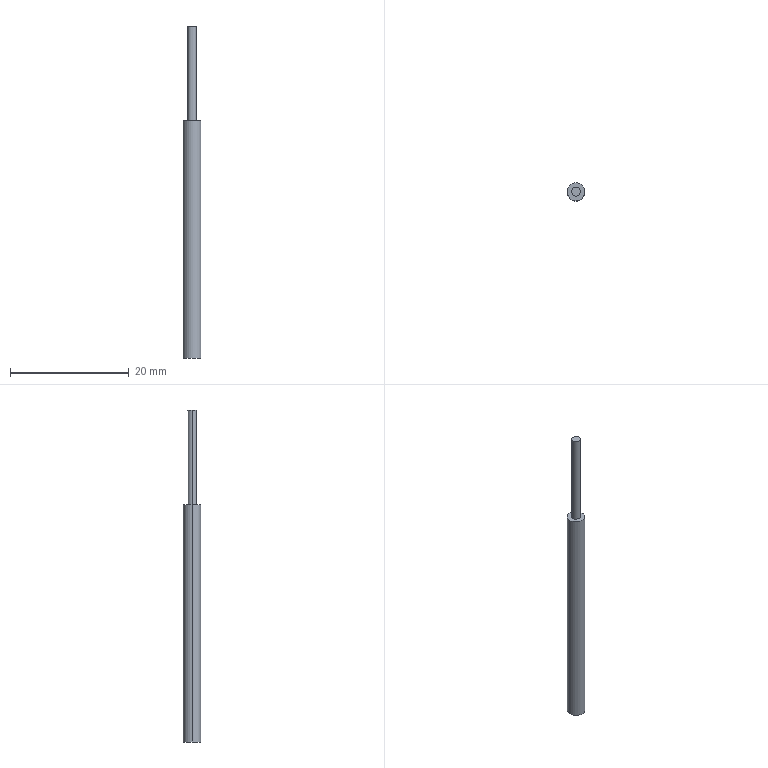Part | SolidWorks | features Extrusion 1, ICE 1 | 1 solid | 7 faces | box 3 x 3 x 56 mm | volume 311.018 mm3 | cylinder 4 | plane 3 | commonest cylinder face diameters 1.5 x2 3 x2
STEP:
#1=CARTESIAN_POINT('',(0.75,0.,56.));
#2=VERTEX_POINT('',#1);
#3=CARTESIAN_POINT('',(-0.75,0.,56.));
#4=VERTEX_POINT('',#3);
#5=CARTESIAN_POINT('',(0.,0.,56.));
#6=DIRECTION('',(0.,0.,1.));
#7=DIRECTION('',(1.,0.,0.));
#8=AXIS2_PLACEMENT_3D('',#5,#6,#7);
#9=CIRCLE('',#8,0.75);
#10=EDGE_CURVE('',#2,#4,#9,.T.);
#11=ORIENTED_EDGE('',*,*,#10,.F.);
#12=CARTESIAN_POINT('',(0.75,0.,40.));
#13=VERTEX_POINT('',#12);
#14=CARTESIAN_POINT('',(0.75,0.,56.));
#15=DIRECTION('',(0.,0.,-1.));
#16=VECTOR('',#15,1000.);
#17=LINE('',#14,#16);
#18=EDGE_CURVE('',#2,#13,#17,.T.);
#19=ORIENTED_EDGE('',*,*,#18,.T.);
#20=CARTESIAN_POINT('',(-0.75,0.,40.));
#21=VERTEX_POINT('',#20);
#22=CARTESIAN_POINT('',(0.,0.,40.));
#23=DIRECTION('',(0.,0.,1.));
#24=DIRECTION('',(1.,0.,0.));
#25=AXIS2_PLACEMENT_3D('',#22,#23,#24);
#26=CIRCLE('',#25,0.75);
#27=EDGE_CURVE('',#13,#21,#26,.T.);
#28=ORIENTED_EDGE('',*,*,#27,.T.);
#29=CARTESIAN_POINT('',(-0.75,0.,56.));
#30=DIRECTION('',(0.,0.,-1.));
#31=VECTOR('',#30,1000.);
#32=LINE('',#29,#31);
#33=EDGE_CURVE('',#4,#21,#32,.T.);
#34=ORIENTED_EDGE('',*,*,#33,.F.);
#35=EDGE_LOOP('',(#11,#19,#28,#34));
#36=FACE_OUTER_BOUND('',#35,.T.);
#37=CARTESIAN_POINT('',(0.,0.,56.));
#38=DIRECTION('',(0.,0.,-1.));
#39=DIRECTION('',(-1.,0.,0.));
#40=AXIS2_PLACEMENT_3D('',#37,#38,#39);
#41=CYLINDRICAL_SURFACE('',#40,0.75);
#42=ADVANCED_FACE('',(#36),#41,.T.);
#43=CARTESIAN_POINT('',(1.5,0.,40.));
#44=VERTEX_POINT('',#43);
#45=CARTESIAN_POINT('',(-1.5,0.,40.));
#46=VERTEX_POINT('',#45);
#47=CARTESIAN_POINT('',(0.,0.,40.));
#48=DIRECTION('',(0.,0.,1.));
#49=DIRECTION('',(1.,0.,0.));
#50=AXIS2_PLACEMENT_3D('',#47,#48,#49);
#51=CIRCLE('',#50,1.5);
#52=EDGE_CURVE('',#44,#46,#51,.T.);
#53=ORIENTED_EDGE('',*,*,#52,.F.);
#54=CARTESIAN_POINT('',(1.5,0.,0.));
#55=VERTEX_POINT('',#54);
#56=CARTESIAN_POINT('',(1.5,0.,40.));
#57=DIRECTION('',(0.,0.,-1.));
#58=VECTOR('',#57,1000.);
#59=LINE('',#56,#58);
#60=EDGE_CURVE('',#44,#55,#59,.T.);
#61=ORIENTED_EDGE('',*,*,#60,.T.);
#62=CARTESIAN_POINT('',(-1.5,0.,0.));
#63=VERTEX_POINT('',#62);
#64=CARTESIAN_POINT('',(0.,0.,0.));
#65=DIRECTION('',(0.,0.,1.));
#66=DIRECTION('',(1.,0.,0.));
#67=AXIS2_PLACEMENT_3D('',#64,#65,#66);
#68=CIRCLE('',#67,1.5);
#69=EDGE_CURVE('',#55,#63,#68,.T.);
#70=ORIENTED_EDGE('',*,*,#69,.T.);
#71=CARTESIAN_POINT('',(-1.5,0.,40.));
#72=DIRECTION('',(0.,0.,-1.));
#73=VECTOR('',#72,1000.);
#74=LINE('',#71,#73);
#75=EDGE_CURVE('',#46,#63,#74,.T.);
#76=ORIENTED_EDGE('',*,*,#75,.F.);
#77=EDGE_LOOP('',(#53,#61,#70,#76));
#78=FACE_OUTER_BOUND('',#77,.T.);
#79=CARTESIAN_POINT('',(0.,0.,40.));
#80=DIRECTION('',(0.,0.,-1.));
#81=DIRECTION('',(-1.,0.,0.));
#82=AXIS2_PLACEMENT_3D('',#79,#80,#81);
#83=CYLINDRICAL_SURFACE('',#82,1.5);
#84=ADVANCED_FACE('',(#78),#83,.T.);
#85=CARTESIAN_POINT('',(0.,0.,40.));
#86=DIRECTION('',(0.,0.,1.));
#87=DIRECTION('',(1.,0.,0.));
#88=AXIS2_PLACEMENT_3D('',#85,#86,#87);
#89=CIRCLE('',#88,1.5);
#90=EDGE_CURVE('',#46,#44,#89,.T.);
#91=ORIENTED_EDGE('',*,*,#90,.T.);
#92=ORIENTED_EDGE('',*,*,#52,.T.);
#93=EDGE_LOOP('',(#91,#92));
#94=FACE_OUTER_BOUND('',#93,.T.);
#95=CARTESIAN_POINT('',(0.,0.,40.));
#96=DIRECTION('',(0.,0.,1.));
#97=DIRECTION('',(1.,0.,0.));
#98=AXIS2_PLACEMENT_3D('',#95,#96,#97);
#99=CIRCLE('',#98,0.75);
#100=EDGE_CURVE('',#21,#13,#99,.T.);
#101=ORIENTED_EDGE('',*,*,#100,.F.);
#102=ORIENTED_EDGE('',*,*,#27,.F.);
#103=EDGE_LOOP('',(#101,#102));
#104=FACE_BOUND('',#103,.T.);
#105=CARTESIAN_POINT('',(0.,0.,40.));
#106=DIRECTION('',(0.,0.,1.));
#107=DIRECTION('',(1.,0.,0.));
#108=AXIS2_PLACEMENT_3D('',#105,#106,#107);
#109=PLANE('',#108);
#110=ADVANCED_FACE('',(#94,#104),#109,.T.);
#111=ORIENTED_EDGE('',*,*,#60,.F.);
#112=ORIENTED_EDGE('',*,*,#90,.F.);
#113=ORIENTED_EDGE('',*,*,#75,.T.);
#114=CARTESIAN_POINT('',(0.,0.,0.));
#115=DIRECTION('',(0.,0.,1.));
#116=DIRECTION('',(1.,0.,0.));
#117=AXIS2_PLACEMENT_3D('',#114,#115,#116);
#118=CIRCLE('',#117,1.5);
#119=EDGE_CURVE('',#63,#55,#118,.T.);
#120=ORIENTED_EDGE('',*,*,#119,.T.);
#121=EDGE_LOOP('',(#111,#112,#113,#120));
#122=FACE_OUTER_BOUND('',#121,.T.);
#123=CARTESIAN_POINT('',(0.,0.,40.));
#124=DIRECTION('',(0.,0.,-1.));
#125=DIRECTION('',(-1.,0.,0.));
#126=AXIS2_PLACEMENT_3D('',#123,#124,#125);
#127=CYLINDRICAL_SURFACE('',#126,1.5);
#128=ADVANCED_FACE('',(#122),#127,.T.);
#129=ORIENTED_EDGE('',*,*,#119,.F.);
#130=ORIENTED_EDGE('',*,*,#69,.F.);
#131=EDGE_LOOP('',(#129,#130));
#132=FACE_OUTER_BOUND('',#131,.T.);
#133=CARTESIAN_POINT('',(0.,0.,0.));
#134=DIRECTION('',(0.,0.,1.));
#135=DIRECTION('',(1.,0.,0.));
#136=AXIS2_PLACEMENT_3D('',#133,#134,#135);
#137=PLANE('',#136);
#138=ADVANCED_FACE('',(#132),#137,.F.);
#139=ORIENTED_EDGE('',*,*,#18,.F.);
#140=CARTESIAN_POINT('',(0.,0.,56.));
#141=DIRECTION('',(0.,0.,1.));
#142=DIRECTION('',(1.,0.,0.));
#143=AXIS2_PLACEMENT_3D('',#140,#141,#142);
#144=CIRCLE('',#143,0.75);
#145=EDGE_CURVE('',#4,#2,#144,.T.);
#146=ORIENTED_EDGE('',*,*,#145,.F.);
#147=ORIENTED_EDGE('',*,*,#33,.T.);
#148=ORIENTED_EDGE('',*,*,#100,.T.);
#149=EDGE_LOOP('',(#139,#146,#147,#148));
#150=FACE_OUTER_BOUND('',#149,.T.);
#151=CARTESIAN_POINT('',(0.,0.,56.));
#152=DIRECTION('',(0.,0.,-1.));
#153=DIRECTION('',(-1.,0.,0.));
#154=AXIS2_PLACEMENT_3D('',#151,#152,#153);
#155=CYLINDRICAL_SURFACE('',#154,0.75);
#156=ADVANCED_FACE('',(#150),#155,.T.);
#157=ORIENTED_EDGE('',*,*,#145,.T.);
#158=ORIENTED_EDGE('',*,*,#10,.T.);
#159=EDGE_LOOP('',(#157,#158));
#160=FACE_OUTER_BOUND('',#159,.T.);
#161=CARTESIAN_POINT('',(0.,0.,56.));
#162=DIRECTION('',(0.,0.,1.));
#163=DIRECTION('',(1.,0.,0.));
#164=AXIS2_PLACEMENT_3D('',#161,#162,#163);
#165=PLANE('',#164);
#166=ADVANCED_FACE('',(#160),#165,.T.);
#167=CLOSED_SHELL('',(#42,#84,#110,#128,#138,#156,#166));
#168=MANIFOLD_SOLID_BREP('',#167);
#169=CARTESIAN_POINT('',(0.,0.,0.));
#170=DIRECTION('',(0.,0.,1.));
#171=DIRECTION('',(1.,0.,0.));
#172=AXIS2_PLACEMENT_3D('',#169,#170,#171);
#173=(LENGTH_UNIT()NAMED_UNIT(*)SI_UNIT(.MILLI.,.METRE.));
#174=UNCERTAINTY_MEASURE_WITH_UNIT(LENGTH_MEASURE(0.00001),#173,'','');
#175=(NAMED_UNIT(*)PLANE_ANGLE_UNIT()SI_UNIT($,.RADIAN.));
#176=(NAMED_UNIT(*)SI_UNIT($,.STERADIAN.)SOLID_ANGLE_UNIT());
#177=(GEOMETRIC_REPRESENTATION_CONTEXT(3)GLOBAL_UNCERTAINTY_ASSIGNED_CONTEXT((#174))GLOBAL_UNIT_ASSIGNED_CONTEXT((#173,#175,#176))REPRESENTATION_CONTEXT('',''));
#178=ADVANCED_BREP_SHAPE_REPRESENTATION('',(#168,#172),#177);